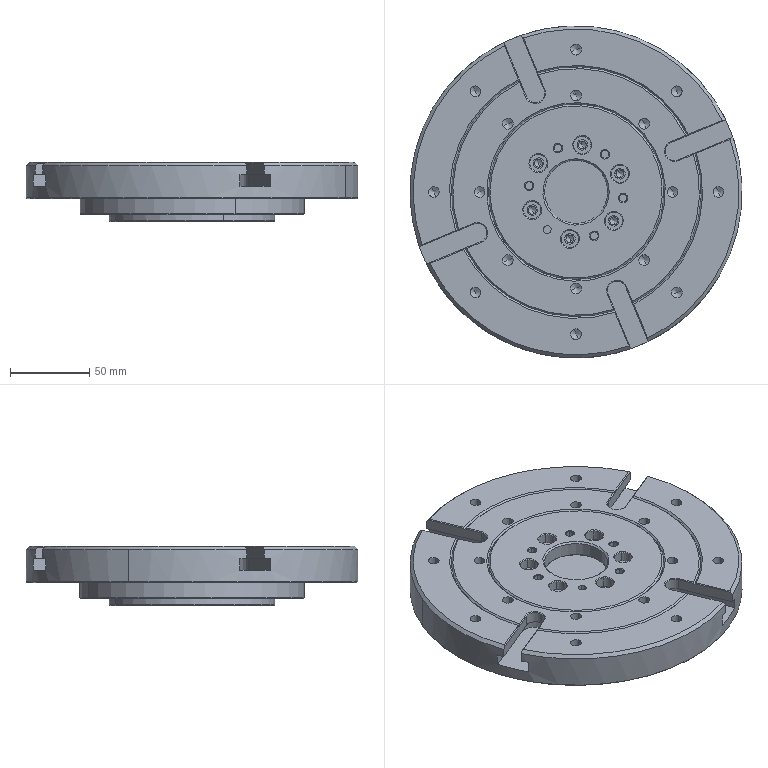NC program | Mastercam | posted with a generic post
Lines 960 to 1884 of 19401:
(25 BNOS |TOOL - 1|DIA. OFF. - 1|LEN. - 1|TOOL DIA. - 25.)
N1986 T1 M6
N1988 G0 G54 G90 X3.794 Y47.619 C0. B180. S3500 M3
N1990 G43 H1 Z34.355
N1992 Z14.355
N1994 G1 Z9.355 F2000.
N1996 X-6.848 Y37.048
N1998 X-6.771 Y36.971
N2000 X-6.317 Y36.476
N2002 X-6.246 Y36.395
N2004 X-5.825 Y35.872
N2006 X-5.759 Y35.786
N2008 X-5.372 Y35.238
N2010 X-5.312 Y35.148
N2012 X-4.961 Y34.576
N2014 X-4.907 Y34.482
N2016 X-4.593 Y33.889
N2018 X-4.545 Y33.792
N2020 X-4.27 Y33.179
N2022 X-4.228 Y33.079
N2024 X-3.994 Y32.451
N2026 X-3.958 Y32.348
N2028 X-3.764 Y31.706
N2030 X-3.735 Y31.602
N2032 X-3.583 Y30.948
N2034 X-3.56 Y30.842
N2036 X-3.45 Y30.18
N2038 X-3.435 Y30.073
N2040 X-3.367 Y29.405
N2042 X-3.359 Y29.297
N2044 X-3.334 Y28.627
N2046 X-3.332 Y28.518
N2048 Y8.518
N2050 X-3.351 Y7.848
N2052 X-3.356 Y7.739
N2054 X-3.418 Y7.071
N2056 X-3.43 Y6.963
N2058 X-3.534 Y6.301
N2060 X-3.553 Y6.194
N2062 X-3.7 Y5.539
N2064 X-3.726 Y5.434
N2066 X-3.914 Y4.79
N2068 X-3.946 Y4.686
N2070 X-4.176 Y4.056
N2072 X-4.215 Y3.954
N2074 X-4.484 Y3.34
N2076 X-4.529 Y3.241
N2078 X-4.837 Y2.645
N2080 X-4.889 Y2.55
N2082 X-5.234 Y1.975
N2084 X-5.292 Y1.883
N2086 X-5.674 Y1.331
N2088 X-5.737 Y1.243
N2090 X-6.154 Y.717
N2092 X-6.222 Y.633
N2094 X-6.672 Y.135
N2096 X-6.746 Y.055
N2098 X-7.226 Y-.413
N2100 X-7.305 Y-.488
N2102 X-7.814 Y-.924
N2104 X-7.898 Y-.993
N2106 X-8.434 Y-1.396
N2108 X-8.522 Y-1.46
N2110 X-9.083 Y-1.828
N2112 X-9.175 Y-1.886
N2114 X-9.853 Y-2.269
N2116 X-10.555 Y-2.608
N2118 X-11.278 Y-2.901
N2120 X-12.017 Y-3.148
N2122 X-12.771 Y-3.346
N2124 X-13.536 Y-3.496
N2126 X-14.309 Y-3.596
N2128 X-15.086 Y-3.646
N2130 X-15.757 Y-3.648
N2132 X-28.857 Y-3.647
N2134 X-29.635 Y-3.598
N2136 X-30.408 Y-3.499
N2138 X-31.173 Y-3.35
N2140 X-31.927 Y-3.153
N2142 X-32.667 Y-2.908
N2144 X-33.39 Y-2.616
N2146 X-34.092 Y-2.278
N2148 X-34.771 Y-1.896
N2150 X-35.425 Y-1.471
N2152 X-36.05 Y-1.005
N2154 X-36.643 Y-.5
N2156 X-37.203 Y.042
N2158 X-37.728 Y.619
N2160 X-38.214 Y1.228
N2162 X-38.66 Y1.867
N2164 X-39.064 Y2.534
N2166 X-39.425 Y3.225
N2168 X-39.74 Y3.937
N2170 X-40.01 Y4.669
N2172 X-40.232 Y5.416
N2174 X-40.405 Y6.176
N2176 X-40.53 Y6.945
N2178 X-40.604 Y7.721
N2180 X-40.629 Y8.5
N2182 Y28.5
N2184 X-40.612 Y29.134
N2186 X-40.606 Y29.243
N2188 X-40.547 Y29.911
N2190 X-40.533 Y30.019
N2192 X-40.431 Y30.682
N2194 X-40.411 Y30.788
N2196 X-40.267 Y31.444
N2198 X-40.24 Y31.549
N2200 X-40.054 Y32.193
N2202 X-40.02 Y32.297
N2204 X-39.794 Y32.928
N2206 X-39.753 Y33.029
N2208 X-39.486 Y33.644
N2210 X-39.44 Y33.742
N2212 X-39.134 Y34.339
N2214 X-39.081 Y34.434
N2216 X-38.738 Y35.011
N2218 X-38.679 Y35.102
N2220 X-38.299 Y35.655
N2222 X-38.235 Y35.742
N2224 X-37.82 Y36.27
N2226 X-37.75 Y36.353
N2228 X-37.303 Y36.853
N2230 X-37.228 Y36.931
N2232 X-36.75 Y37.401
N2234 X-36.67 Y37.475
N2236 X-36.162 Y37.913
N2238 X-36.077 Y37.982
N2240 X-35.543 Y38.387
N2242 X-35.454 Y38.449
N2244 X-34.894 Y38.819
N2246 X-34.802 Y38.876
N2248 X-34.22 Y39.209
N2250 X-34.124 Y39.26
N2252 X-33.521 Y39.556
N2254 X-33.422 Y39.6
N2256 X-32.802 Y39.856
N2258 X-32.701 Y39.894
N2260 X-32.066 Y40.11
N2262 X-31.962 Y40.142
N2264 X-31.314 Y40.316
N2266 X-31.208 Y40.341
N2268 X-30.551 Y40.474
N2270 X-30.444 Y40.492
N2272 X-29.779 Y40.582
N2274 X-29.671 Y40.594
N2276 X-29.002 Y40.641
N2278 X-28.893 Y40.645
N2280 X-28.222 Y40.65
N2282 X-15.231
N2284 X-15.123 Y40.647
N2286 X-14.453 Y40.608
N2288 X-14.345 Y40.599
N2290 X-13.679 Y40.517
N2292 X-13.572 Y40.501
N2294 X-12.912 Y40.377
N2296 X-12.806 Y40.354
N2298 X-12.156 Y40.187
N2300 X-12.052 Y40.157
N2302 X-11.414 Y39.95
N2304 X-11.312 Y39.913
N2306 X-10.688 Y39.665
N2308 X-10.589 Y39.622
N2310 X-9.983 Y39.335
N2312 X-9.886 Y39.286
N2314 X-9.299 Y38.96
N2316 X-9.206 Y38.905
N2318 X-8.642 Y38.542
N2320 X-8.552 Y38.481
N2322 X-8.012 Y38.082
N2324 X-7.926 Y38.016
N2326 X-7.413 Y37.584
N2328 X-7.332 Y37.512
N2330 X-6.848 Y37.048
N2332 X-6.676 Y36.867
N2334 X-6.563 Y36.745
N2336 X-6.157 Y36.286 Z9.354
N2338 X-6.053 Y36.157
N2340 X-5.677 Y35.673
N2342 X-5.581 Y35.538 Z9.353
N2344 X-5.237 Y35.031
N2346 X-5.15 Y34.889
N2348 X-4.839 Y34.361 Z9.352
N2350 X-4.761 Y34.214
N2352 X-4.484 Y33.668 Z9.351
N2354 X-4.416 Y33.516
N2356 X-4.175 Y32.953 Z9.35
N2358 X-4.117 Y32.797
N2360 X-3.912 Y32.22
N2362 X-3.864 Y32.061
N2364 X-3.697 Y31.471 Z9.349
N2366 X-3.659 Y31.309
N2368 X-3.53 Y30.71 Z9.348
N2370 X-3.503 Y30.547
N2372 X-3.412 Y29.94 Z9.347
N2374 X-3.395 Y29.775
N2376 X-3.344 Y29.165
N2378 X-3.338 Y28.999 Z9.346
N2380 X-3.322 Y28.386
N2382 X-3.304 Y8.336 Z9.325
N2384 X-3.324 Y7.723
N2386 X-3.338 Y7.557
N2388 X-3.398 Y6.946 Z9.324
N2390 X-3.423 Y6.781
N2392 X-3.522 Y6.175 Z9.323
N2394 X-3.557 Y6.012
N2396 X-3.694 Y5.414 Z9.322
N2398 X-3.74 Y5.254
N2400 X-3.915 Y4.665
N2402 X-3.971 Y4.508 Z9.321
N2404 X-4.184 Y3.932
N2406 X-4.249 Y3.779
N2408 X-4.498 Y3.218 Z9.32
N2410 X-4.573 Y3.069
N2412 X-4.858 Y2.525 Z9.319
N2414 X-4.942 Y2.382
N2416 X-5.262 Y1.857 Z9.318
N2418 X-5.355 Y1.719
N2420 X-5.707 Y1.216
N2422 X-5.809 Y1.084
N2424 X-6.192 Y.604 Z9.317
N2426 X-6.302 Y.48
N2428 X-6.716 Y.025 Z9.316
N2430 X-6.834 Y-.092
N2432 X-7.276 Y-.519 Z9.315
N2434 X-7.401 Y-.629
N2436 X-7.869 Y-1.026
N2438 X-8. Y-1.128 Z9.314
N2440 X-8.493 Y-1.494
N2442 X-8.631 Y-1.588
N2444 X-9.146 Y-1.922 Z9.313
N2446 X-9.29 Y-2.006
N2448 X-9.826 Y-2.307 Z9.312
N2450 X-9.974 Y-2.381
N2452 X-10.681 Y-2.712 Z9.311
N2454 X-11.408 Y-2.998 Z9.31
N2456 X-12.151 Y-3.236
N2458 X-12.908 Y-3.426 Z9.309
N2460 X-13.676 Y-3.567 Z9.308
N2462 X-14.451 Y-3.659 Z9.307
N2464 X-15.23 Y-3.701 Z9.306
N2466 X-28.167 Y-3.716 Z9.293
N2468 X-28.949 Y-3.711
N2470 X-29.729 Y-3.657 Z9.292
N2472 X-30.503 Y-3.553 Z9.291
N2474 X-31.27 Y-3.399 Z9.29
N2476 X-32.025 Y-3.197 Z9.289
N2478 X-32.765 Y-2.947
N2480 X-33.489 Y-2.651 Z9.288
N2482 X-34.191 Y-2.309 Z9.287
N2484 X-34.871 Y-1.922 Z9.286
N2486 X-35.524 Y-1.493 Z9.285
N2488 X-36.149 Y-1.023
N2490 X-36.742 Y-.514 Z9.284
N2492 X-37.301 Y.032 Z9.283
N2494 X-37.825 Y.612 Z9.282
N2496 X-38.31 Y1.225 Z9.281
N2498 X-38.756 Y1.867
N2500 X-39.159 Y2.537 Z9.28
N2502 X-39.519 Y3.231 Z9.279
N2504 X-39.834 Y3.947 Z9.278
N2506 X-40.102 Y4.681
N2508 X-40.323 Y5.431 Z9.277
N2510 X-40.496 Y6.193 Z9.276
N2512 X-40.619 Y6.965 Z9.275
N2514 X-40.693 Y7.743 Z9.274
N2516 X-40.718 Y8.525
N2518 X-40.74 Y28.476 Z9.253
N2520 X-40.736 Y28.775
N2522 X-40.731 Y28.933
N2524 X-40.694 Y29.548 Z9.252
N2526 X-40.679 Y29.715
N2528 X-40.603 Y30.326
N2530 X-40.578 Y30.491 Z9.251
N2532 X-40.463 Y31.097
N2534 X-40.427 Y31.26
N2536 X-40.273 Y31.857 Z9.25
N2538 X-40.227 Y32.017
N2540 X-40.036 Y32.603 Z9.249
N2542 X-39.98 Y32.76
N2544 X-39.751 Y33.333 Z9.248
N2546 X-39.685 Y33.486
N2548 X-39.421 Y34.043
N2550 X-39.345 Y34.191 Z9.247
N2552 X-39.046 Y34.73
N2554 X-38.96 Y34.874
N2556 X-38.627 Y35.392 Z9.246
N2558 X-38.533 Y35.53
N2560 X-38.168 Y36.026 Z9.245
N2562 X-38.065 Y36.158
N2564 X-37.668 Y36.63 Z9.244
N2566 X-37.557 Y36.755
N2568 X-37.132 Y37.2
N2570 X-37.013 Y37.318 Z9.243
N2572 X-36.56 Y37.735
N2574 X-36.434 Y37.845
N2576 X-35.955 Y38.233 Z9.242
N2578 X-35.822 Y38.334
N2580 X-35.319 Y38.69 Z9.241
N2582 X-35.181 Y38.783
N2584 X-34.656 Y39.107 Z9.24
N2586 X-34.512 Y39.191
N2588 X-33.967 Y39.48
N2590 X-33.818 Y39.555 Z9.239
N2592 X-33.256 Y39.809
N2594 X-33.102 Y39.874
N2596 X-32.526 Y40.091 Z9.238
N2598 X-32.368 Y40.146
N2600 X-31.779 Y40.327 Z9.237
N2602 X-31.618 Y40.371
N2604 X-31.018 Y40.514 Z9.236
N2606 X-30.855 Y40.548
N2608 X-30.247 Y40.652
N2610 X-30.082 Y40.676
N2612 X-29.469 Y40.741 Z9.235
N2614 X-29.303 Y40.755
N2616 X-28.687 Y40.781 Z9.234
N2618 X-28.52 Y40.784
N2620 X-15.538 Y40.798 Z9.221
N2622 X-14.921 Y40.785 Z9.22
N2624 X-14.754 Y40.777
N2626 X-14.139 Y40.725 Z9.219
N2628 X-13.973 Y40.707
N2630 X-13.362 Y40.615
N2632 X-13.198 Y40.586 Z9.218
N2634 X-12.594 Y40.456
N2636 X-12.432 Y40.417
N2638 X-11.838 Y40.248 Z9.217
N2640 X-11.678 Y40.199
N2642 X-11.097 Y39.993 Z9.216
N2644 X-10.94 Y39.934
N2646 X-10.373 Y39.691 Z9.215
N2648 X-10.221 Y39.622
N2650 X-9.67 Y39.343
N2652 X-9.522 Y39.264
N2654 X-8.991 Y38.951 Z9.214
N2656 X-8.848 Y38.863
N2658 X-8.337 Y38.517 Z9.213
N2660 X-8.201 Y38.42
N2662 X-7.713 Y38.042 Z9.212
N2664 X-7.583 Y37.937
N2666 X-7.121 Y37.528
N2668 X-6.998 Y37.415 Z9.211
N2670 X-6.739 Y37.155
N2672 X-6.321 Y36.713 Z9.21
N2674 X-5.816 Y36.113
N2676 X-5.35 Y35.482 Z9.209
N2678 X-4.926 Y34.823 Z9.208
N2680 X-4.544 Y34.139 Z9.207
N2682 X-4.207 Y33.431 Z9.206
N2684 X-3.915 Y32.703
N2686 X-3.671 Y31.958 Z9.205
N2688 X-3.474 Y31.199 Z9.204
N2690 X-3.326 Y30.43 Z9.203
N2692 X-3.227 Y29.652 Z9.202
N2694 X-3.178 Y28.869
N2696 X-3.162 Y8.158 Z9.181
N2698 X-3.208 Y7.374 Z9.18
N2700 X-3.304 Y6.595 Z9.179
N2702 X-3.449 Y5.824 Z9.178
N2704 X-3.643 Y5.063
N2706 X-3.885 Y4.316 Z9.177
N2708 X-4.175 Y3.586 Z9.176
N2710 X-4.51 Y2.876 Z9.175
N2712 X-4.889 Y2.189 Z9.174
N2714 X-5.312 Y1.528
N2716 X-5.776 Y.894 Z9.173
N2718 X-6.279 Y.291 Z9.172
N2720 X-6.819 Y-.278 Z9.171
N2722 X-7.395 Y-.812
N2724 X-8.003 Y-1.308 Z9.17
N2726 X-8.642 Y-1.765 Z9.169
N2728 X-9.308 Y-2.18 Z9.168
N2730 X-10. Y-2.551 Z9.167
N2732 X-10.714 Y-2.878
N2734 X-11.447 Y-3.159 Z9.166
N2736 X-12.196 Y-3.393 Z9.165
N2738 X-12.959 Y-3.579 Z9.164
N2740 X-13.732 Y-3.715 Z9.163
N2742 X-14.512 Y-3.803
N2744 X-15.297 Y-3.841 Z9.162
N2746 X-28.254 Y-3.85 Z9.149
N2748 X-29.04 Y-3.839 Z9.148
N2750 X-29.824 Y-3.779 Z9.147
N2752 X-30.602 Y-3.669 Z9.146
N2754 X-31.371 Y-3.51
N2756 X-32.129 Y-3.302 Z9.145
N2758 X-32.872 Y-3.047 Z9.144
N2760 X-33.597 Y-2.744 Z9.143
N2762 X-34.302 Y-2.397 Z9.142
N2764 X-34.983 Y-2.005
N2766 X-35.638 Y-1.57 Z9.141
N2768 X-36.264 Y-1.095 Z9.14
N2770 X-36.859 Y-.581 Z9.139
N2772 X-37.419 Y-.03
N2774 X-37.944 Y.555 Z9.138
N2776 X-38.43 Y1.172 Z9.137
N2778 X-38.876 Y1.819 Z9.136
N2780 X-39.28 Y2.493 Z9.135
N2782 X-39.64 Y3.192
N2784 X-39.955 Y3.912 Z9.134
N2786 X-40.224 Y4.65 Z9.133
N2788 X-40.446 Y5.404 Z9.132
N2790 X-40.619 Y6.171 Z9.131
N2792 X-40.743 Y6.947
N2794 X-40.817 Y7.729 Z9.13
N2796 X-40.842 Y8.515 Z9.129
N2798 X-40.856 Y28.485 Z9.109
N2800 X-40.832 Y29.254 Z9.108
N2802 X-40.76 Y30.037 Z9.107
N2804 X-40.638 Y30.815
N2806 X-40.467 Y31.582 Z9.106
N2808 X-40.247 Y32.338 Z9.105
N2810 X-39.98 Y33.078 Z9.104
N2812 X-39.667 Y33.8 Z9.103
N2814 X-39.308 Y34.5
N2816 X-38.906 Y35.176 Z9.102
N2818 X-38.461 Y35.825 Z9.101
N2820 X-37.976 Y36.445 Z9.1
N2822 X-37.453 Y37.033 Z9.099
N2824 X-36.894 Y37.586
N2826 X-36.3 Y38.102 Z9.098
N2828 X-35.675 Y38.58 Z9.097
N2830 X-35.021 Y39.017 Z9.096
N2832 X-34.34 Y39.412
N2834 X-33.636 Y39.763 Z9.095
N2836 X-32.91 Y40.068 Z9.094
N2838 X-32.167 Y40.327 Z9.093
N2840 X-31.409 Y40.538 Z9.092
N2842 X-30.639 Y40.7
N2844 X-29.861 Y40.814 Z9.091
N2846 X-29.076 Y40.877 Z9.09
N2848 X-28.362 Y40.891 Z9.089
N2850 X-15.304 Y40.9 Z9.076
N2852 X-14.517 Y40.864 Z9.075
N2854 X-13.734 Y40.779
N2856 X-12.958 Y40.643 Z9.074
N2858 X-12.193 Y40.459 Z9.073
N2860 X-11.44 Y40.226 Z9.072
N2862 X-10.704 Y39.947 Z9.071
N2864 X-9.987 Y39.621
N2866 X-9.292 Y39.25 Z9.07
N2868 X-8.622 Y38.836 Z9.069
N2870 X-7.98 Y38.38 Z9.068
N2872 X-7.368 Y37.884 Z9.067
N2874 X-6.789 Y37.351
N2876 X-6.667 Y37.224 Z9.066
N2878 X-6.174 Y36.698
N2880 X-5.672 Y36.091 Z9.065
N2882 X-5.21 Y35.453 Z9.064
N2884 X-4.79 Y34.788 Z9.063
N2886 X-4.412 Y34.097
N2888 X-4.079 Y33.384 Z9.062
N2890 X-3.792 Y32.651 Z9.061
N2892 X-3.552 Y31.901 Z9.06
N2894 X-3.36 Y31.137 Z9.059
N2896 X-3.217 Y30.363
N2898 X-3.123 Y29.582 Z9.058
N2900 X-3.079 Y28.796 Z9.057
N2902 X-3.07 Y8.736 Z9.037
N2904 X-3.074 Y8.05 Z9.036
N2906 X-3.127 Y7.264 Z9.035
N2908 X-3.23 Y6.483
N2910 X-3.383 Y5.71 Z9.034
N2912 X-3.584 Y4.948 Z9.033
N2914 X-3.832 Y4.2 Z9.032
N2916 X-4.128 Y3.47 Z9.031
N2918 X-4.47 Y2.76
N2920 X-4.855 Y2.073 Z9.03
N2922 X-5.284 Y1.412 Z9.029
N2924 X-5.754 Y.779 Z9.028
N2926 X-6.263 Y.177
N2928 X-6.808 Y-.391 Z9.027
N2930 X-7.389 Y-.923 Z9.026
N2932 X-8.003 Y-1.418 Z9.025
N2934 X-8.646 Y-1.872 Z9.024
N2936 X-9.317 Y-2.285
N2938 X-10.013 Y-2.655 Z9.023
N2940 X-10.731 Y-2.98 Z9.022
N2942 X-11.468 Y-3.258 Z9.021
N2944 X-12.222 Y-3.489 Z9.02
N2946 X-12.988 Y-3.672
N2948 X-13.764 Y-3.807 Z9.019
N2950 X-14.548 Y-3.891 Z9.018
N2952 X-15.335 Y-3.927 Z9.017
N2954 X-28.307 Y-3.932 Z9.004
N2956 X-29.095 Y-3.918 Z9.003
N2958 X-29.881 Y-3.854
N2960 X-30.661 Y-3.74 Z9.002
N2962 X-31.433 Y-3.578 Z9.001
N2964 X-32.192 Y-3.366 Z9.
N2966 X-32.937 Y-3.107
N2968 X-33.663 Y-2.801 Z8.999
N2970 X-34.369 Y-2.45 Z8.998
N2972 X-35.051 Y-2.055 Z8.997
N2974 X-35.707 Y-1.618 Z8.996
N2976 X-36.334 Y-1.139
N2978 X-36.929 Y-.622 Z8.995
N2980 X-37.49 Y-.069 Z8.994
N2982 X-38.016 Y.519 Z8.993
N2984 X-38.502 Y1.14 Z8.992
N2986 X-38.949 Y1.789
N2988 X-39.353 Y2.466 Z8.991
N2990 X-39.714 Y3.167 Z8.99
N2992 X-40.029 Y3.89 Z8.989
N2994 X-40.298 Y4.631 Z8.988
N2996 X-40.52 Y5.387
N2998 X-40.693 Y6.157 Z8.987
N3000 X-40.818 Y6.935 Z8.986
N3002 X-40.892 Y7.72 Z8.985
N3004 X-40.917 Y8.508 Z8.984
N3006 X-40.923 Y28.658 Z8.964
N3008 X-40.92 Y28.755
N3010 X-40.889 Y29.441
N3012 X-40.879 Y29.543 Z8.963
N3014 X-40.805 Y30.225
N3016 X-40.789 Y30.326
N3018 X-40.671 Y31.003 Z8.962
N3020 X-40.649 Y31.103
N3022 X-40.488 Y31.77 Z8.961
N3024 X-40.46 Y31.868
N3026 X-40.257 Y32.524 Z8.96
N3028 X-40.222 Y32.621
N3030 X-39.979 Y33.263
N3032 X-39.938 Y33.357 Z8.959
N3034 X-39.655 Y33.982
N3036 X-39.608 Y34.073
N3038 X-39.285 Y34.679 Z8.958
N3040 X-39.233 Y34.767
N3042 X-38.872 Y35.351 Z8.957
N3044 X-38.815 Y35.436
N3046 X-38.418 Y35.996 Z8.956
N3048 X-38.355 Y36.077
N3050 X-37.924 Y36.611
N3052 X-37.855 Y36.687 Z8.955
N3054 X-37.391 Y37.193
N3056 X-37.318 Y37.265
N3058 X-36.823 Y37.74 Z8.954
N3060 X-36.746 Y37.808
N3062 X-36.221 Y38.251 Z8.953
N3064 X-36.14 Y38.313
N3066 X-35.588 Y38.722 Z8.952
N3068 X-35.503 Y38.779
N3070 X-34.927 Y39.152
N3072 X-34.839 Y39.203
N3074 X-34.24 Y39.539 Z8.951
N3076 X-34.148 Y39.585
N3078 X-33.529 Y39.882 Z8.95
N3080 X-33.435 Y39.922
N3082 X-32.799 Y40.18 Z8.949
N3084 X-32.702 Y40.214
N3086 X-32.051 Y40.43 Z8.948
N3088 X-31.952 Y40.458
N3090 X-31.288 Y40.633
N3092 X-31.188 Y40.654
N3094 X-30.514 Y40.787 Z8.947
N3096 X-30.413 Y40.802
N3098 X-29.732 Y40.892 Z8.946
N3100 X-29.63 Y40.9
N3102 X-28.945 Y40.947 Z8.945
N3104 X-28.156 Y40.953
N3106 X-15.168 Y40.957 Z8.932
N3108 X-14.38 Y40.913 Z8.931
N3110 X-13.596 Y40.818 Z8.93
N3112 X-12.82 Y40.674 Z8.929
N3114 X-12.055 Y40.481 Z8.928
N3116 X-11.303 Y40.24
N3118 X-10.568 Y39.953 Z8.927
N3120 X-9.853 Y39.619 Z8.926
N3122 X-9.16 Y39.24 Z8.925
N3124 X-8.493 Y38.818 Z8.924
N3126 X-7.853 Y38.355
N3128 X-7.245 Y37.853 Z8.923
N3130 X-6.669 Y37.313 Z8.922
N3132 X-6.624 Y37.265
N3134 X-6.106 Y36.71 Z8.921
N3136 X-5.605 Y36.1 Z8.92
N3138 X-5.144 Y35.461
N3140 X-4.725 Y34.793 Z8.919
N3142 X-4.348 Y34.1 Z8.918
N3144 X-4.016 Y33.385 Z8.917
N3146 X-3.73 Y32.65 Z8.916
N3148 X-3.491 Y31.899
N3150 X-3.3 Y31.134 Z8.915
N3152 X-3.157 Y30.358 Z8.914
N3154 X-3.064 Y29.575 Z8.913
N3156 X-3.021 Y28.788
N3158 X-3.015 Y8.809 Z8.893
N3160 X-3.02 Y8.024 Z8.892
N3162 X-3.075 Y7.237 Z8.891
N3164 X-3.179 Y6.455 Z8.89
N3166 X-3.333 Y5.681 Z8.889
N3168 X-3.536 Y4.919
N3170 X-3.786 Y4.171 Z8.888
N3172 X-4.083 Y3.44 Z8.887
N3174 X-4.425 Y2.729 Z8.886
N3176 X-4.812 Y2.042 Z8.885
N3178 X-5.242 Y1.38
N3180 X-5.712 Y.747 Z8.884
N3182 X-6.222 Y.145 Z8.883
N3184 X-6.769 Y-.424 Z8.882
N3186 X-7.351 Y-.956 Z8.881
N3188 X-7.965 Y-1.451
N3190 X-8.609 Y-1.907 Z8.88
N3192 X-9.281 Y-2.32 Z8.879
N3194 X-10.02 Y-2.711 Z8.878
N3196 X-10.741 Y-3.035 Z8.877
N3198 X-11.48 Y-3.312
N3200 X-12.235 Y-3.542 Z8.876
N3202 X-13.003 Y-3.723 Z8.875
N3204 X-13.781 Y-3.856 Z8.874
N3206 X-14.566 Y-3.939
N3208 X-15.354 Y-3.973 Z8.873
N3210 X-28.334 Y-3.975 Z8.86
N3212 X-29.124 Y-3.959 Z8.859
N3214 X-29.911 Y-3.894 Z8.858
N3216 X-30.692 Y-3.778 Z8.857
N3218 X-31.464 Y-3.614
N3220 X-32.224 Y-3.4 Z8.856
N3222 X-32.969 Y-3.14 Z8.855
N3224 X-33.697 Y-2.832 Z8.854
N3226 X-34.403 Y-2.48 Z8.853
N3228 X-35.1 Y-2.075
N3230 X-35.755 Y-1.636 Z8.852
N3232 X-36.382 Y-1.156 Z8.851
N3234 X-36.977 Y-.638 Z8.85
N3236 X-37.538 Y-.083 Z8.849
N3238 X-38.063 Y.506
N3240 X-38.55 Y1.127 Z8.848
N3242 X-38.996 Y1.778 Z8.847
N3244 X-39.401 Y2.455 Z8.846
N3246 X-39.761 Y3.157 Z8.845
N3248 X-40.077 Y3.88
N3250 X-40.346 Y4.622 Z8.844
N3252 X-40.568 Y5.38 Z8.843
N3254 X-40.741 Y6.149 Z8.842
N3256 X-40.866 Y6.929
N3258 X-40.94 Y7.714 Z8.841
N3260 X-40.966 Y8.503 Z8.84
N3262 X-40.971 Y28.4 Z8.82
N3264 X-40.97 Y28.687
N3266 X-40.934 Y29.473 Z8.819
N3268 X-40.847 Y30.257 Z8.818
N3270 X-40.712 Y31.035 Z8.817
N3272 X-40.527 Y31.803
N3274 X-40.294 Y32.557 Z8.816
N3276 X-40.014 Y33.295 Z8.815
N3278 X-39.688 Y34.014 Z8.814
N3280 X-39.317 Y34.711 Z8.813
N3282 X-38.903 Y35.382
N3284 X-38.447 Y36.027 Z8.812
N3286 X-37.951 Y36.641 Z8.811
N3288 X-37.417 Y37.223 Z8.81
N3290 X-36.847 Y37.769
N3292 X-36.244 Y38.279 Z8.809
N3294 X-35.61 Y38.749 Z8.808
N3296 X-34.948 Y39.178 Z8.807
N3298 X-34.259 Y39.565 Z8.806
N3300 X-34.196 Y39.598
N3302 X-33.483 Y39.937 Z8.805
N3304 X-32.75 Y40.231
N3306 X-31.999 Y40.478 Z8.804
N3308 X-31.235 Y40.677 Z8.803
N3310 X-30.459 Y40.827 Z8.802
N3312 X-29.676 Y40.928
N3314 X-28.888 Y40.979 Z8.801
N3316 X-28.578 Y40.981 Z8.8
N3318 X-15.109 Y40.983 Z8.787
N3320 X-14.32 Y40.934 Z8.786
N3322 X-13.536 Y40.836 Z8.785
N3324 X-12.76 Y40.688
N3326 X-11.995 Y40.491 Z8.784
N3328 X-11.243 Y40.247 Z8.783
N3330 X-10.509 Y39.955 Z8.782
N3332 X-9.794 Y39.618 Z8.781
N3334 X-9.109 Y39.241
N3336 X-8.442 Y38.818 Z8.78
N3338 X-7.803 Y38.354 Z8.779
N3340 X-7.195 Y37.85 Z8.778
N3342 X-6.62 Y37.309 Z8.777
N3344 X-6.6 Y37.287
N3346 X-6.066 Y36.716
N3348 X-5.566 Y36.107 Z8.776
N3350 X-5.105 Y35.467 Z8.775
N3352 X-4.685 Y34.799 Z8.774
N3354 X-4.308 Y34.106
N3356 X-3.976 Y33.391 Z8.773
N3358 X-3.69 Y32.656 Z8.772
N3360 X-3.45 Y31.904 Z8.771
N3362 X-3.259 Y31.139 Z8.77
N3364 X-3.116 Y30.363
N3366 X-3.023 Y29.58 Z8.769
N3368 X-2.979 Y28.793 Z8.768
N3370 X-2.973 Y8.805 Z8.748
N3372 X-2.979 Y8.024 Z8.747
N3374 X-3.034 Y7.237 Z8.746
N3376 X-3.139 Y6.455
N3378 X-3.292 Y5.681 Z8.745
N3380 X-3.495 Y4.918 Z8.744
N3382 X-3.745 Y4.17 Z8.743
N3384 X-4.042 Y3.439 Z8.742
N3386 X-4.384 Y2.729
N3388 X-4.771 Y2.041 Z8.741
N3390 X-5.201 Y1.379 Z8.74
N3392 X-5.671 Y.746 Z8.739
N3394 X-6.181 Y.144
N3396 X-6.727 Y-.425 Z8.738
N3398 X-7.309 Y-.958 Z8.737
N3400 X-7.923 Y-1.454 Z8.736
N3402 X-8.567 Y-1.909 Z8.735
N3404 X-9.246 Y-2.327
N3406 X-10.007 Y-2.731 Z8.734
N3408 X-10.726 Y-3.053 Z8.733
N3410 X-11.466 Y-3.331 Z8.732
N3412 X-12.221 Y-3.561 Z8.731
N3414 X-12.99 Y-3.743
N3416 X-13.768 Y-3.876 Z8.73
N3418 X-14.554 Y-3.959 Z8.729
N3420 X-15.343 Y-3.993 Z8.728
N3422 X-28.344 Y-3.994 Z8.715
N3424 X-29.15 Y-3.976 Z8.714
N3426 X-29.937 Y-3.909
N3428 X-30.718 Y-3.793 Z8.713
N3430 X-31.491 Y-3.627 Z8.712
N3432 X-32.251 Y-3.413 Z8.711
N3434 X-32.997 Y-3.151 Z8.71
N3436 X-33.724 Y-2.843
N3438 X-34.461 Y-2.472 Z8.709
N3440 X-35.136 Y-2.08 Z8.708
N3442 X-35.792 Y-1.641 Z8.707
N3444 X-36.419 Y-1.161 Z8.706
N3446 X-37.014 Y-.643
N3448 X-37.576 Y-.088 Z8.705
N3450 X-38.101 Y.501 Z8.704
N3452 X-38.587 Y1.122 Z8.703
N3454 X-39.034 Y1.773
N3456 X-39.439 Y2.45 Z8.702
N3458 X-39.799 Y3.152 Z8.701
N3460 X-40.115 Y3.876 Z8.7
N3462 X-40.385 Y4.617 Z8.699
N3464 X-40.607 Y5.375
N3466 X-40.78 Y6.145 Z8.698
N3468 X-40.905 Y6.924 Z8.697
N3470 X-40.98 Y7.709 Z8.696
N3472 X-41.005 Y8.498 Z8.695
N3474 X-41.011 Y28.286 Z8.676
N3476 X-41.01 Y28.687 Z8.675
N3478 X-40.973 Y29.47 Z8.674
N3480 X-40.887 Y30.254
N3482 X-40.752 Y31.032 Z8.673
N3484 X-40.567 Y31.8 Z8.672
N3486 X-40.335 Y32.554 Z8.671
N3488 X-40.055 Y33.292
N3490 X-39.729 Y34.011 Z8.67
N3492 X-39.358 Y34.708 Z8.669
N3494 X-38.944 Y35.38 Z8.668
N3496 X-38.488 Y36.025 Z8.667
N3498 X-37.992 Y36.639
N3500 X-37.459 Y37.221 Z8.666
N3502 X-36.889 Y37.768 Z8.665
N3504 X-36.286 Y38.277 Z8.664
N3506 X-35.653 Y38.748 Z8.663
N3508 X-34.983 Y39.182
N3510 X-34.301 Y39.565 Z8.662
N3512 X-34.196 Y39.62
N3514 X-33.484 Y39.957 Z8.661
N3516 X-32.75 Y40.25 Z8.66
N3518 X-31.999 Y40.496 Z8.659
N3520 X-31.233 Y40.694
N3522 X-30.457 Y40.843 Z8.658
N3524 X-29.673 Y40.942 Z8.657
N3526 X-28.883 Y40.992 Z8.656
N3528 X-15.069 Y40.993 Z8.642
N3530 X-14.281 Y40.943
N3532 X-13.496 Y40.843 Z8.641
N3534 X-12.72 Y40.694 Z8.64
N3536 X-11.955 Y40.496 Z8.639
N3538 X-11.204 Y40.25 Z8.638
N3540 X-10.47 Y39.957
N3542 X-9.755 Y39.618 Z8.637
N3544 X-9.074 Y39.243 Z8.636
N3546 X-8.407 Y38.82 Z8.635
N3548 X-7.768 Y38.356
N3550 X-7.159 Y37.853 Z8.634
N3552 X-6.584 Y37.312 Z8.633
N3554 X-6.579 Y37.307
N3556 X-6.568 Y37.295
N3558 X-6.03 Y36.718 Z8.632
N3560 X-5.529 Y36.109 Z8.631
N3562 X-5.068 Y35.469
N3564 X-4.648 Y34.801 Z8.63
N3566 X-4.271 Y34.108 Z8.629
N3568 X-3.938 Y33.393 Z8.628
N3570 X-3.652 Y32.658 Z8.627
N3572 X-3.412 Y31.907
N3574 X-3.221 Y31.142 Z8.626
N3576 X-3.078 Y30.366 Z8.625
N3578 X-2.985 Y29.583 Z8.624
N3580 X-2.941 Y28.795 Z8.623
N3582 X-2.935 Y8.802 Z8.604
N3584 X-2.941 Y8.026 Z8.603
N3586 X-2.995 Y7.238 Z8.602
N3588 X-3.1 Y6.456 Z8.601
N3590 X-3.253 Y5.683 Z8.6
N3592 X-3.455 Y4.92
N3594 X-3.706 Y4.172 Z8.599
N3596 X-4.002 Y3.441 Z8.598
N3598 X-4.345 Y2.73 Z8.597
N3600 X-4.732 Y2.042 Z8.596
N3602 X-5.161 Y1.38
N3604 X-5.631 Y.747 Z8.595
N3606 X-6.141 Y.145 Z8.594
N3608 X-6.688 Y-.424 Z8.593
N3610 X-7.269 Y-.957 Z8.592
N3612 X-7.883 Y-1.453
N3614 X-8.527 Y-1.908 Z8.591
N3616 X-9.21 Y-2.329 Z8.59
N3618 X-9.971 Y-2.732 Z8.589
N3620 X-10.686 Y-3.054 Z8.588
N3622 X-11.425 Y-3.332
N3624 X-12.18 Y-3.563 Z8.587
N3626 X-12.948 Y-3.745 Z8.586
N3628 X-13.727 Y-3.879 Z8.585
N3630 X-14.512 Y-3.964
N3632 X-15.301 Y-3.998 Z8.584
N3634 X-28.346 Y-3.999 Z8.571
N3636 X-29.186 Y-3.981 Z8.57
N3638 X-29.973 Y-3.914 Z8.569
N3640 X-30.754 Y-3.796 Z8.568
N3642 X-31.527 Y-3.63
N3644 X-32.287 Y-3.416 Z8.567
N3646 X-33.032 Y-3.154 Z8.566
N3648 X-33.759 Y-2.845 Z8.565
N3650 X-34.5 Y-2.472 Z8.564
N3652 X-35.172 Y-2.082
N3654 X-35.828 Y-1.643 Z8.563
N3656 X-36.455 Y-1.163 Z8.562
N3658 X-37.05 Y-.645 Z8.561
N3660 X-37.612 Y-.091 Z8.56
N3662 X-38.137 Y.498
N3664 X-38.624 Y1.119 Z8.559
N3666 X-39.071 Y1.77 Z8.558
N3668 X-39.475 Y2.447 Z8.557
N3670 X-39.836 Y3.149 Z8.556
N3672 X-40.152 Y3.872
N3674 X-40.422 Y4.614 Z8.555
N3676 X-40.644 Y5.371 Z8.554
N3678 X-40.818 Y6.141 Z8.553
N3680 X-40.943 Y6.92 Z8.552
N3682 X-41.018 Y7.706
N3684 X-41.044 Y8.495 Z8.551
N3686 X-41.05 Y28.172 Z8.531
N3688 X-41.048 Y28.687
N3690 X-41.012 Y29.466 Z8.53
N3692 X-40.926 Y30.251 Z8.529
N3694 X-40.791 Y31.029 Z8.528
N3696 X-40.607 Y31.796
N3698 X-40.374 Y32.551 Z8.527
N3700 X-40.095 Y33.289 Z8.526
N3702 X-39.769 Y34.008 Z8.525
N3704 X-39.398 Y34.705 Z8.524
N3706 X-38.984 Y35.377
N3708 X-38.529 Y36.022 Z8.523
N3710 X-38.033 Y36.636 Z8.522
N3712 X-37.5 Y37.218 Z8.521
N3714 X-36.931 Y37.765
N3716 X-36.328 Y38.275 Z8.52
N3718 X-35.694 Y38.746 Z8.519
N3720 X-35.021 Y39.182 Z8.518
N3722 X-34.342 Y39.563 Z8.517
N3724 X-34.235 Y39.62
N3726 X-33.526 Y39.956 Z8.516
N3728 X-32.792 Y40.249
N3730 X-32.041 Y40.495 Z8.515
N3732 X-31.276 Y40.693 Z8.514
N3734 X-30.5 Y40.843 Z8.513
N3736 X-29.716 Y40.943
N3738 X-28.921 Y40.994 Z8.512
N3740 X-15.035 Y40.993 Z8.498
N3742 X-14.246 Y40.943 Z8.497
N3744 X-13.462 Y40.844 Z8.496
N3746 X-12.686 Y40.695
N3748 X-11.921 Y40.497 Z8.495
N3750 X-11.169 Y40.251 Z8.494
N3752 X-10.435 Y39.958 Z8.493
N3754 X-9.721 Y39.62 Z8.492
N3756 X-9.039 Y39.245
N3758 X-8.372 Y38.823 Z8.491
N3760 X-7.733 Y38.359 Z8.49
N3762 X-7.124 Y37.856 Z8.489
N3764 X-6.561 Y37.326 Z8.488
N3766 X-6.533 Y37.298
N3768 X-5.994 Y36.722
N3770 X-5.493 Y36.112 Z8.487
N3772 X-5.032 Y35.473 Z8.486
N3774 X-4.611 Y34.805 Z8.485
N3776 X-4.234 Y34.112 Z8.484
N3778 X-3.902 Y33.397
N3780 X-3.615 Y32.663 Z8.483
N3782 X-3.375 Y31.911 Z8.482
N3784 X-3.183 Y31.146 Z8.481
N3786 X-3.04 Y30.37
N3788 X-2.946 Y29.587 Z8.48
N3790 X-2.902 Y28.8 Z8.479
N3792 X-2.896 Y8.802 Z8.459
N3794 X-2.902 Y8.03 Z8.458
N3796 X-2.956 Y7.243 Z8.457
N3798 X-3.06 Y6.461
N3800 X-3.214 Y5.687 Z8.456
N3802 X-3.416 Y4.924 Z8.455
N3804 X-3.665 Y4.176 Z8.454
N3806 X-3.962 Y3.445
N3808 X-4.304 Y2.734 Z8.453
N3810 X-4.691 Y2.046 Z8.452
N3812 X-5.12 Y1.384 Z8.451
N3814 X-5.59 Y.751 Z8.45
N3816 X-6.099 Y.148
N3818 X-6.646 Y-.421 Z8.449
N3820 X-7.227 Y-.954 Z8.448
N3822 X-7.841 Y-1.45 Z8.447
N3824 X-8.485 Y-1.906 Z8.446
N3826 X-9.171 Y-2.329
N3828 X-9.932 Y-2.732 Z8.445
N3830 X-10.643 Y-3.052 Z8.444
N3832 X-11.382 Y-3.33 Z8.443